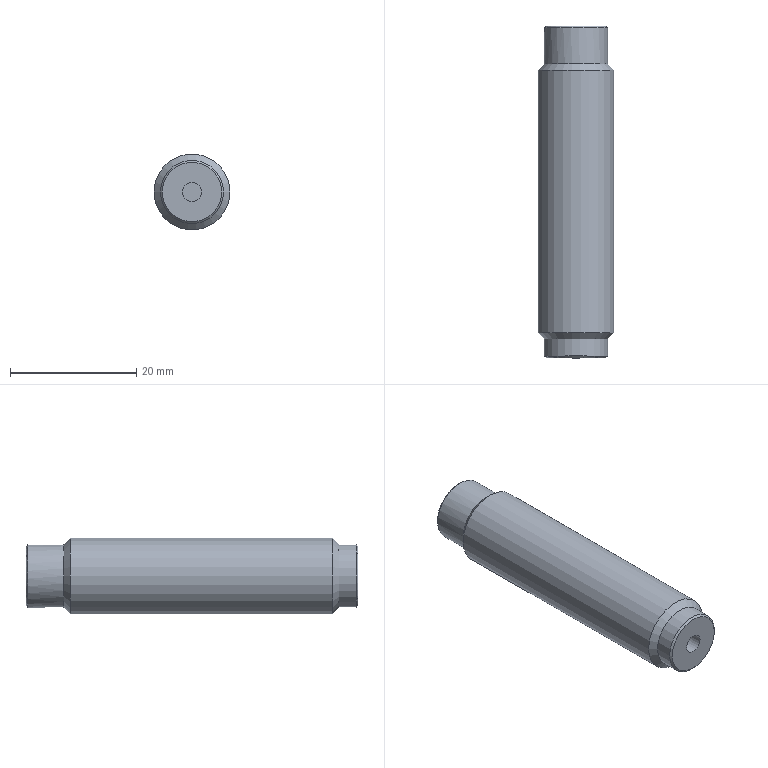Part | NX | features BODY_5003_027_C-AC1210S-N_1 2 | 1 solid | 11 faces | box 12 x 52.5 x 12 mm | volume 5489 mm3 | cylinder 4 | cone 4 | plane 3 | commonest cylinder face diameters 10 x2 3 x1 12 x1
STEP:
#1=CARTESIAN_POINT('',(127.525,3.402,-122.));
#2=VERTEX_POINT('',#1);
#3=CARTESIAN_POINT('',(121.525,3.402,-122.));
#4=DIRECTION('',(0.,-1.,0.));
#5=DIRECTION('',(1.,0.,0.));
#6=AXIS2_PLACEMENT_3D('',#3,#4,#5);
#7=CIRCLE('',#6,6.);
#8=EDGE_CURVE('',#2,#2,#7,.F.);
#9=ORIENTED_EDGE('',*,*,#8,.T.);
#10=EDGE_LOOP('',(#9));
#11=FACE_BOUND('',#10,.T.);
#12=CARTESIAN_POINT('',(127.525,44.902,-122.));
#13=VERTEX_POINT('',#12);
#14=CARTESIAN_POINT('',(121.525,44.902,-122.));
#15=DIRECTION('',(0.,-1.,0.));
#16=DIRECTION('',(1.,0.,0.));
#17=AXIS2_PLACEMENT_3D('',#14,#15,#16);
#18=CIRCLE('',#17,6.);
#19=EDGE_CURVE('',#13,#13,#18,.T.);
#20=ORIENTED_EDGE('',*,*,#19,.T.);
#21=EDGE_LOOP('',(#20));
#22=FACE_BOUND('',#21,.T.);
#23=CARTESIAN_POINT('',(121.525,-3.223,-122.));
#24=DIRECTION('',(0.,-1.,0.));
#25=DIRECTION('',(1.,0.,0.));
#26=AXIS2_PLACEMENT_3D('',#23,#24,#25);
#27=CYLINDRICAL_SURFACE('',#26,6.);
#28=ADVANCED_FACE('',(#11,#22),#27,.T.);
#29=ORIENTED_EDGE('',*,*,#8,.F.);
#30=EDGE_LOOP('',(#29));
#31=FACE_BOUND('',#30,.T.);
#32=CARTESIAN_POINT('',(116.525,2.402,-122.));
#33=VERTEX_POINT('',#32);
#34=CARTESIAN_POINT('',(121.525,2.402,-122.));
#35=DIRECTION('',(0.,1.,0.));
#36=DIRECTION('',(-1.,0.,0.));
#37=AXIS2_PLACEMENT_3D('',#34,#35,#36);
#38=CIRCLE('',#37,5.);
#39=EDGE_CURVE('',#33,#33,#38,.T.);
#40=ORIENTED_EDGE('',*,*,#39,.T.);
#41=EDGE_LOOP('',(#40));
#42=FACE_BOUND('',#41,.T.);
#43=CARTESIAN_POINT('',(121.525,3.402,-122.));
#44=DIRECTION('',(0.,1.,0.));
#45=DIRECTION('',(-1.,0.,0.));
#46=AXIS2_PLACEMENT_3D('',#43,#44,#45);
#47=CONICAL_SURFACE('',#46,6.,0.7854);
#48=ADVANCED_FACE('',(#31,#42),#47,.T.);
#49=ORIENTED_EDGE('',*,*,#19,.F.);
#50=EDGE_LOOP('',(#49));
#51=FACE_BOUND('',#50,.T.);
#52=CARTESIAN_POINT('',(126.525,45.902,-122.));
#53=VERTEX_POINT('',#52);
#54=CARTESIAN_POINT('',(121.525,45.902,-122.));
#55=DIRECTION('',(0.,-1.,0.));
#56=DIRECTION('',(1.,0.,0.));
#57=AXIS2_PLACEMENT_3D('',#54,#55,#56);
#58=CIRCLE('',#57,5.);
#59=EDGE_CURVE('',#53,#53,#58,.T.);
#60=ORIENTED_EDGE('',*,*,#59,.T.);
#61=EDGE_LOOP('',(#60));
#62=FACE_BOUND('',#61,.T.);
#63=CARTESIAN_POINT('',(121.525,44.902,-122.));
#64=DIRECTION('',(0.,-1.,0.));
#65=DIRECTION('',(1.,0.,0.));
#66=AXIS2_PLACEMENT_3D('',#63,#64,#65);
#67=CONICAL_SURFACE('',#66,6.,0.7854);
#68=ADVANCED_FACE('',(#51,#62),#67,.T.);
#69=CARTESIAN_POINT('',(126.525,-0.2978,-122.));
#70=VERTEX_POINT('',#69);
#71=CARTESIAN_POINT('',(121.525,-0.2978,-122.));
#72=DIRECTION('',(0.,-1.,0.));
#73=DIRECTION('',(1.,0.,0.));
#74=AXIS2_PLACEMENT_3D('',#71,#72,#73);
#75=CIRCLE('',#74,5.);
#76=EDGE_CURVE('',#70,#70,#75,.F.);
#77=ORIENTED_EDGE('',*,*,#76,.T.);
#78=EDGE_LOOP('',(#77));
#79=FACE_BOUND('',#78,.T.);
#80=ORIENTED_EDGE('',*,*,#39,.F.);
#81=EDGE_LOOP('',(#80));
#82=FACE_BOUND('',#81,.T.);
#83=CARTESIAN_POINT('',(121.525,-3.223,-122.));
#84=DIRECTION('',(0.,-1.,0.));
#85=DIRECTION('',(1.,0.,0.));
#86=AXIS2_PLACEMENT_3D('',#83,#84,#85);
#87=CYLINDRICAL_SURFACE('',#86,5.);
#88=ADVANCED_FACE('',(#79,#82),#87,.T.);
#89=ORIENTED_EDGE('',*,*,#59,.F.);
#90=EDGE_LOOP('',(#89));
#91=FACE_BOUND('',#90,.T.);
#92=CARTESIAN_POINT('',(126.525,51.602,-122.));
#93=VERTEX_POINT('',#92);
#94=CARTESIAN_POINT('',(121.525,51.602,-122.));
#95=DIRECTION('',(0.,-1.,0.));
#96=DIRECTION('',(1.,0.,0.));
#97=AXIS2_PLACEMENT_3D('',#94,#95,#96);
#98=CIRCLE('',#97,5.);
#99=EDGE_CURVE('',#93,#93,#98,.T.);
#100=ORIENTED_EDGE('',*,*,#99,.T.);
#101=EDGE_LOOP('',(#100));
#102=FACE_BOUND('',#101,.T.);
#103=CARTESIAN_POINT('',(121.525,-3.223,-122.));
#104=DIRECTION('',(0.,-1.,0.));
#105=DIRECTION('',(1.,0.,0.));
#106=AXIS2_PLACEMENT_3D('',#103,#104,#105);
#107=CYLINDRICAL_SURFACE('',#106,5.);
#108=ADVANCED_FACE('',(#91,#102),#107,.T.);
#109=ORIENTED_EDGE('',*,*,#76,.F.);
#110=EDGE_LOOP('',(#109));
#111=FACE_BOUND('',#110,.T.);
#112=CARTESIAN_POINT('',(116.825,-0.5978,-122.));
#113=VERTEX_POINT('',#112);
#114=CARTESIAN_POINT('',(121.525,-0.5978,-122.));
#115=DIRECTION('',(0.,1.,0.));
#116=DIRECTION('',(-1.,0.,0.));
#117=AXIS2_PLACEMENT_3D('',#114,#115,#116);
#118=CIRCLE('',#117,4.7);
#119=EDGE_CURVE('',#113,#113,#118,.T.);
#120=ORIENTED_EDGE('',*,*,#119,.T.);
#121=EDGE_LOOP('',(#120));
#122=FACE_BOUND('',#121,.T.);
#123=CARTESIAN_POINT('',(121.525,-0.2978,-122.));
#124=DIRECTION('',(0.,1.,0.));
#125=DIRECTION('',(-1.,0.,0.));
#126=AXIS2_PLACEMENT_3D('',#123,#124,#125);
#127=CONICAL_SURFACE('',#126,5.,0.7854);
#128=ADVANCED_FACE('',(#111,#122),#127,.T.);
#129=ORIENTED_EDGE('',*,*,#99,.F.);
#130=EDGE_LOOP('',(#129));
#131=FACE_BOUND('',#130,.T.);
#132=CARTESIAN_POINT('',(121.525,51.902,-126.7));
#133=VERTEX_POINT('',#132);
#134=CARTESIAN_POINT('',(121.525,51.902,-122.));
#135=DIRECTION('',(0.,-1.,0.));
#136=DIRECTION('',(0.,0.,-1.));
#137=AXIS2_PLACEMENT_3D('',#134,#135,#136);
#138=CIRCLE('',#137,4.7);
#139=EDGE_CURVE('',#133,#133,#138,.T.);
#140=ORIENTED_EDGE('',*,*,#139,.T.);
#141=EDGE_LOOP('',(#140));
#142=FACE_BOUND('',#141,.T.);
#143=CARTESIAN_POINT('',(121.525,51.602,-122.));
#144=DIRECTION('',(0.,-1.,0.));
#145=DIRECTION('',(0.,0.,-1.));
#146=AXIS2_PLACEMENT_3D('',#143,#144,#145);
#147=CONICAL_SURFACE('',#146,5.,0.7854);
#148=ADVANCED_FACE('',(#131,#142),#147,.T.);
#149=CARTESIAN_POINT('',(123.025,-0.5978,-122.));
#150=VERTEX_POINT('',#149);
#151=CARTESIAN_POINT('',(121.525,-0.5978,-122.));
#152=DIRECTION('',(0.,-1.,0.));
#153=DIRECTION('',(1.,0.,0.));
#154=AXIS2_PLACEMENT_3D('',#151,#152,#153);
#155=CIRCLE('',#154,1.5);
#156=EDGE_CURVE('',#150,#150,#155,.F.);
#157=ORIENTED_EDGE('',*,*,#156,.T.);
#158=EDGE_LOOP('',(#157));
#159=FACE_BOUND('',#158,.T.);
#160=ORIENTED_EDGE('',*,*,#119,.F.);
#161=EDGE_LOOP('',(#160));
#162=FACE_BOUND('',#161,.T.);
#163=CARTESIAN_POINT('',(121.525,-0.5978,-122.));
#164=DIRECTION('',(0.,-1.,0.));
#165=DIRECTION('',(1.,0.,0.));
#166=AXIS2_PLACEMENT_3D('',#163,#164,#165);
#167=PLANE('',#166);
#168=ADVANCED_FACE('',(#159,#162),#167,.T.);
#169=ORIENTED_EDGE('',*,*,#139,.F.);
#170=EDGE_LOOP('',(#169));
#171=FACE_BOUND('',#170,.T.);
#172=CARTESIAN_POINT('',(121.525,51.902,-117.3));
#173=DIRECTION('',(0.,1.,0.));
#174=DIRECTION('',(-1.,0.,0.));
#175=AXIS2_PLACEMENT_3D('',#172,#173,#174);
#176=PLANE('',#175);
#177=ADVANCED_FACE('',(#171),#176,.T.);
#178=ORIENTED_EDGE('',*,*,#156,.F.);
#179=EDGE_LOOP('',(#178));
#180=FACE_BOUND('',#179,.T.);
#181=CARTESIAN_POINT('',(123.025,13.402,-122.));
#182=VERTEX_POINT('',#181);
#183=CARTESIAN_POINT('',(121.525,13.402,-122.));
#184=DIRECTION('',(0.,-1.,0.));
#185=DIRECTION('',(1.,0.,0.));
#186=AXIS2_PLACEMENT_3D('',#183,#184,#185);
#187=CIRCLE('',#186,1.5);
#188=EDGE_CURVE('',#182,#182,#187,.T.);
#189=ORIENTED_EDGE('',*,*,#188,.F.);
#190=EDGE_LOOP('',(#189));
#191=FACE_BOUND('',#190,.T.);
#192=CARTESIAN_POINT('',(121.525,-3.223,-122.));
#193=DIRECTION('',(0.,-1.,0.));
#194=DIRECTION('',(1.,0.,0.));
#195=AXIS2_PLACEMENT_3D('',#192,#193,#194);
#196=CYLINDRICAL_SURFACE('',#195,1.5);
#197=ADVANCED_FACE('',(#180,#191),#196,.F.);
#198=ORIENTED_EDGE('',*,*,#188,.T.);
#199=EDGE_LOOP('',(#198));
#200=FACE_BOUND('',#199,.T.);
#201=CARTESIAN_POINT('',(121.525,13.402,-122.));
#202=DIRECTION('',(0.,-1.,0.));
#203=DIRECTION('',(1.,0.,0.));
#204=AXIS2_PLACEMENT_3D('',#201,#202,#203);
#205=PLANE('',#204);
#206=ADVANCED_FACE('',(#200),#205,.T.);
#207=CLOSED_SHELL('',(#28,#48,#68,#88,#108,#128,#148,#168,#177,#197,#206));
#208=MANIFOLD_SOLID_BREP('',#207);
#209=(LENGTH_UNIT()NAMED_UNIT(*)SI_UNIT(.MILLI.,.METRE.));
#210=UNCERTAINTY_MEASURE_WITH_UNIT(LENGTH_MEASURE(0.00001),#209,'','');
#211=(NAMED_UNIT(*)PLANE_ANGLE_UNIT()SI_UNIT($,.RADIAN.));
#212=(NAMED_UNIT(*)SI_UNIT($,.STERADIAN.)SOLID_ANGLE_UNIT());
#213=(GEOMETRIC_REPRESENTATION_CONTEXT(3)GLOBAL_UNCERTAINTY_ASSIGNED_CONTEXT((#210))GLOBAL_UNIT_ASSIGNED_CONTEXT((#209,#211,#212))REPRESENTATION_CONTEXT('',''));
#214=ADVANCED_BREP_SHAPE_REPRESENTATION('',(#208),#213);